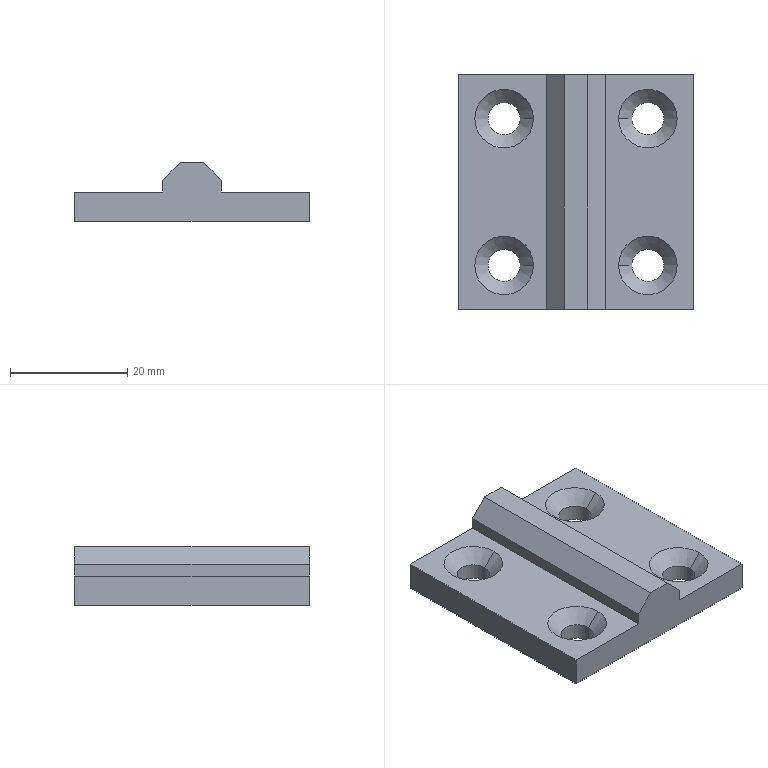Part | STEP file | Hinge bracket 40-40 | 1 solid | 28 faces | box 40 x 40 x 10 mm | volume 8942 mm3 | plane 12 | cone 8 | cylinder 8 | commonest cylinder face diameters 5.5 x8
STEP:
#1=CARTESIAN_POINT('',(-15.,12.5,2.75));
#2=VERTEX_POINT('',#1);
#3=CARTESIAN_POINT('',(-9.5,12.5,2.75));
#4=VERTEX_POINT('',#3);
#5=CARTESIAN_POINT('',(-12.25,12.5,2.75));
#6=DIRECTION('',(0.,0.,1.));
#7=DIRECTION('',(1.,0.,0.));
#8=AXIS2_PLACEMENT_3D('',#5,#6,#7);
#9=CIRCLE('',#8,2.75);
#10=EDGE_CURVE('',#2,#4,#9,.T.);
#11=ORIENTED_EDGE('',*,*,#10,.F.);
#12=CARTESIAN_POINT('',(-17.25,12.5,5.));
#13=VERTEX_POINT('',#12);
#14=CARTESIAN_POINT('',(-17.25,12.5,5.));
#15=DIRECTION('',(-0.7071,0.,0.7071));
#16=VECTOR('',#15,1000.);
#17=LINE('',#14,#16);
#18=EDGE_CURVE('',#2,#13,#17,.T.);
#19=ORIENTED_EDGE('',*,*,#18,.T.);
#20=CARTESIAN_POINT('',(-7.25,12.5,5.));
#21=VERTEX_POINT('',#20);
#22=CARTESIAN_POINT('',(-12.25,12.5,5.));
#23=DIRECTION('',(0.,0.,1.));
#24=DIRECTION('',(1.,0.,0.));
#25=AXIS2_PLACEMENT_3D('',#22,#23,#24);
#26=CIRCLE('',#25,5.);
#27=EDGE_CURVE('',#13,#21,#26,.T.);
#28=ORIENTED_EDGE('',*,*,#27,.T.);
#29=CARTESIAN_POINT('',(-7.25,12.5,5.));
#30=DIRECTION('',(0.7071,0.,0.7071));
#31=VECTOR('',#30,1000.);
#32=LINE('',#29,#31);
#33=EDGE_CURVE('',#4,#21,#32,.T.);
#34=ORIENTED_EDGE('',*,*,#33,.F.);
#35=EDGE_LOOP('',(#11,#19,#28,#34));
#36=FACE_OUTER_BOUND('',#35,.T.);
#37=CARTESIAN_POINT('',(-12.25,12.5,5.));
#38=DIRECTION('',(0.,0.,1.));
#39=DIRECTION('',(1.,0.,0.));
#40=AXIS2_PLACEMENT_3D('',#37,#38,#39);
#41=CONICAL_SURFACE('',#40,5.,0.7854);
#42=ADVANCED_FACE('',(#36),#41,.F.);
#43=CARTESIAN_POINT('',(-15.,12.5,0.));
#44=VERTEX_POINT('',#43);
#45=CARTESIAN_POINT('',(-9.5,12.5,0.));
#46=VERTEX_POINT('',#45);
#47=CARTESIAN_POINT('',(-12.25,12.5,0.));
#48=DIRECTION('',(0.,0.,1.));
#49=DIRECTION('',(1.,0.,0.));
#50=AXIS2_PLACEMENT_3D('',#47,#48,#49);
#51=CIRCLE('',#50,2.75);
#52=EDGE_CURVE('',#44,#46,#51,.T.);
#53=ORIENTED_EDGE('',*,*,#52,.F.);
#54=CARTESIAN_POINT('',(-15.,12.5,5.));
#55=DIRECTION('',(0.,0.,1.));
#56=VECTOR('',#55,1000.);
#57=LINE('',#54,#56);
#58=EDGE_CURVE('',#44,#2,#57,.T.);
#59=ORIENTED_EDGE('',*,*,#58,.T.);
#60=ORIENTED_EDGE('',*,*,#10,.T.);
#61=CARTESIAN_POINT('',(-9.5,12.5,5.));
#62=DIRECTION('',(0.,0.,1.));
#63=VECTOR('',#62,1000.);
#64=LINE('',#61,#63);
#65=EDGE_CURVE('',#46,#4,#64,.T.);
#66=ORIENTED_EDGE('',*,*,#65,.F.);
#67=EDGE_LOOP('',(#53,#59,#60,#66));
#68=FACE_OUTER_BOUND('',#67,.T.);
#69=CARTESIAN_POINT('',(-12.25,12.5,5.));
#70=DIRECTION('',(0.,0.,1.));
#71=DIRECTION('',(1.,0.,0.));
#72=AXIS2_PLACEMENT_3D('',#69,#70,#71);
#73=CYLINDRICAL_SURFACE('',#72,2.75);
#74=ADVANCED_FACE('',(#68),#73,.F.);
#75=CARTESIAN_POINT('',(-15.,-12.5,2.75));
#76=VERTEX_POINT('',#75);
#77=CARTESIAN_POINT('',(-9.5,-12.5,2.75));
#78=VERTEX_POINT('',#77);
#79=CARTESIAN_POINT('',(-12.25,-12.5,2.75));
#80=DIRECTION('',(0.,0.,1.));
#81=DIRECTION('',(1.,0.,0.));
#82=AXIS2_PLACEMENT_3D('',#79,#80,#81);
#83=CIRCLE('',#82,2.75);
#84=EDGE_CURVE('',#76,#78,#83,.T.);
#85=ORIENTED_EDGE('',*,*,#84,.F.);
#86=CARTESIAN_POINT('',(-17.25,-12.5,5.));
#87=VERTEX_POINT('',#86);
#88=CARTESIAN_POINT('',(-17.25,-12.5,5.));
#89=DIRECTION('',(-0.7071,0.,0.7071));
#90=VECTOR('',#89,1000.);
#91=LINE('',#88,#90);
#92=EDGE_CURVE('',#76,#87,#91,.T.);
#93=ORIENTED_EDGE('',*,*,#92,.T.);
#94=CARTESIAN_POINT('',(-7.25,-12.5,5.));
#95=VERTEX_POINT('',#94);
#96=CARTESIAN_POINT('',(-12.25,-12.5,5.));
#97=DIRECTION('',(0.,0.,1.));
#98=DIRECTION('',(1.,0.,0.));
#99=AXIS2_PLACEMENT_3D('',#96,#97,#98);
#100=CIRCLE('',#99,5.);
#101=EDGE_CURVE('',#87,#95,#100,.T.);
#102=ORIENTED_EDGE('',*,*,#101,.T.);
#103=CARTESIAN_POINT('',(-7.25,-12.5,5.));
#104=DIRECTION('',(0.7071,0.,0.7071));
#105=VECTOR('',#104,1000.);
#106=LINE('',#103,#105);
#107=EDGE_CURVE('',#78,#95,#106,.T.);
#108=ORIENTED_EDGE('',*,*,#107,.F.);
#109=EDGE_LOOP('',(#85,#93,#102,#108));
#110=FACE_OUTER_BOUND('',#109,.T.);
#111=CARTESIAN_POINT('',(-12.25,-12.5,5.));
#112=DIRECTION('',(0.,0.,1.));
#113=DIRECTION('',(1.,0.,0.));
#114=AXIS2_PLACEMENT_3D('',#111,#112,#113);
#115=CONICAL_SURFACE('',#114,5.,0.7854);
#116=ADVANCED_FACE('',(#110),#115,.F.);
#117=CARTESIAN_POINT('',(-15.,-12.5,0.));
#118=VERTEX_POINT('',#117);
#119=CARTESIAN_POINT('',(-9.5,-12.5,0.));
#120=VERTEX_POINT('',#119);
#121=CARTESIAN_POINT('',(-12.25,-12.5,0.));
#122=DIRECTION('',(0.,0.,1.));
#123=DIRECTION('',(1.,0.,0.));
#124=AXIS2_PLACEMENT_3D('',#121,#122,#123);
#125=CIRCLE('',#124,2.75);
#126=EDGE_CURVE('',#118,#120,#125,.T.);
#127=ORIENTED_EDGE('',*,*,#126,.F.);
#128=CARTESIAN_POINT('',(-15.,-12.5,5.));
#129=DIRECTION('',(0.,0.,1.));
#130=VECTOR('',#129,1000.);
#131=LINE('',#128,#130);
#132=EDGE_CURVE('',#118,#76,#131,.T.);
#133=ORIENTED_EDGE('',*,*,#132,.T.);
#134=ORIENTED_EDGE('',*,*,#84,.T.);
#135=CARTESIAN_POINT('',(-9.5,-12.5,5.));
#136=DIRECTION('',(0.,0.,1.));
#137=VECTOR('',#136,1000.);
#138=LINE('',#135,#137);
#139=EDGE_CURVE('',#120,#78,#138,.T.);
#140=ORIENTED_EDGE('',*,*,#139,.F.);
#141=EDGE_LOOP('',(#127,#133,#134,#140));
#142=FACE_OUTER_BOUND('',#141,.T.);
#143=CARTESIAN_POINT('',(-12.25,-12.5,5.));
#144=DIRECTION('',(0.,0.,1.));
#145=DIRECTION('',(1.,0.,0.));
#146=AXIS2_PLACEMENT_3D('',#143,#144,#145);
#147=CYLINDRICAL_SURFACE('',#146,2.75);
#148=ADVANCED_FACE('',(#142),#147,.F.);
#149=CARTESIAN_POINT('',(9.5,-12.5,2.75));
#150=VERTEX_POINT('',#149);
#151=CARTESIAN_POINT('',(15.,-12.5,2.75));
#152=VERTEX_POINT('',#151);
#153=CARTESIAN_POINT('',(12.25,-12.5,2.75));
#154=DIRECTION('',(0.,0.,1.));
#155=DIRECTION('',(1.,0.,0.));
#156=AXIS2_PLACEMENT_3D('',#153,#154,#155);
#157=CIRCLE('',#156,2.75);
#158=EDGE_CURVE('',#150,#152,#157,.T.);
#159=ORIENTED_EDGE('',*,*,#158,.F.);
#160=CARTESIAN_POINT('',(7.25,-12.5,5.));
#161=VERTEX_POINT('',#160);
#162=CARTESIAN_POINT('',(7.25,-12.5,5.));
#163=DIRECTION('',(-0.7071,0.,0.7071));
#164=VECTOR('',#163,1000.);
#165=LINE('',#162,#164);
#166=EDGE_CURVE('',#150,#161,#165,.T.);
#167=ORIENTED_EDGE('',*,*,#166,.T.);
#168=CARTESIAN_POINT('',(17.25,-12.5,5.));
#169=VERTEX_POINT('',#168);
#170=CARTESIAN_POINT('',(12.25,-12.5,5.));
#171=DIRECTION('',(0.,0.,1.));
#172=DIRECTION('',(1.,0.,0.));
#173=AXIS2_PLACEMENT_3D('',#170,#171,#172);
#174=CIRCLE('',#173,5.);
#175=EDGE_CURVE('',#161,#169,#174,.T.);
#176=ORIENTED_EDGE('',*,*,#175,.T.);
#177=CARTESIAN_POINT('',(17.25,-12.5,5.));
#178=DIRECTION('',(0.7071,0.,0.7071));
#179=VECTOR('',#178,1000.);
#180=LINE('',#177,#179);
#181=EDGE_CURVE('',#152,#169,#180,.T.);
#182=ORIENTED_EDGE('',*,*,#181,.F.);
#183=EDGE_LOOP('',(#159,#167,#176,#182));
#184=FACE_OUTER_BOUND('',#183,.T.);
#185=CARTESIAN_POINT('',(12.25,-12.5,5.));
#186=DIRECTION('',(0.,0.,1.));
#187=DIRECTION('',(1.,0.,0.));
#188=AXIS2_PLACEMENT_3D('',#185,#186,#187);
#189=CONICAL_SURFACE('',#188,5.,0.7854);
#190=ADVANCED_FACE('',(#184),#189,.F.);
#191=CARTESIAN_POINT('',(9.5,-12.5,0.));
#192=VERTEX_POINT('',#191);
#193=CARTESIAN_POINT('',(15.,-12.5,0.));
#194=VERTEX_POINT('',#193);
#195=CARTESIAN_POINT('',(12.25,-12.5,0.));
#196=DIRECTION('',(0.,0.,1.));
#197=DIRECTION('',(1.,0.,0.));
#198=AXIS2_PLACEMENT_3D('',#195,#196,#197);
#199=CIRCLE('',#198,2.75);
#200=EDGE_CURVE('',#192,#194,#199,.T.);
#201=ORIENTED_EDGE('',*,*,#200,.F.);
#202=CARTESIAN_POINT('',(9.5,-12.5,5.));
#203=DIRECTION('',(0.,0.,1.));
#204=VECTOR('',#203,1000.);
#205=LINE('',#202,#204);
#206=EDGE_CURVE('',#192,#150,#205,.T.);
#207=ORIENTED_EDGE('',*,*,#206,.T.);
#208=ORIENTED_EDGE('',*,*,#158,.T.);
#209=CARTESIAN_POINT('',(15.,-12.5,5.));
#210=DIRECTION('',(0.,0.,1.));
#211=VECTOR('',#210,1000.);
#212=LINE('',#209,#211);
#213=EDGE_CURVE('',#194,#152,#212,.T.);
#214=ORIENTED_EDGE('',*,*,#213,.F.);
#215=EDGE_LOOP('',(#201,#207,#208,#214));
#216=FACE_OUTER_BOUND('',#215,.T.);
#217=CARTESIAN_POINT('',(12.25,-12.5,5.));
#218=DIRECTION('',(0.,0.,1.));
#219=DIRECTION('',(1.,0.,0.));
#220=AXIS2_PLACEMENT_3D('',#217,#218,#219);
#221=CYLINDRICAL_SURFACE('',#220,2.75);
#222=ADVANCED_FACE('',(#216),#221,.F.);
#223=CARTESIAN_POINT('',(9.5,12.5,2.75));
#224=VERTEX_POINT('',#223);
#225=CARTESIAN_POINT('',(15.,12.5,2.75));
#226=VERTEX_POINT('',#225);
#227=CARTESIAN_POINT('',(12.25,12.5,2.75));
#228=DIRECTION('',(0.,0.,1.));
#229=DIRECTION('',(1.,0.,0.));
#230=AXIS2_PLACEMENT_3D('',#227,#228,#229);
#231=CIRCLE('',#230,2.75);
#232=EDGE_CURVE('',#224,#226,#231,.T.);
#233=ORIENTED_EDGE('',*,*,#232,.F.);
#234=CARTESIAN_POINT('',(7.25,12.5,5.));
#235=VERTEX_POINT('',#234);
#236=CARTESIAN_POINT('',(7.25,12.5,5.));
#237=DIRECTION('',(-0.7071,0.,0.7071));
#238=VECTOR('',#237,1000.);
#239=LINE('',#236,#238);
#240=EDGE_CURVE('',#224,#235,#239,.T.);
#241=ORIENTED_EDGE('',*,*,#240,.T.);
#242=CARTESIAN_POINT('',(17.25,12.5,5.));
#243=VERTEX_POINT('',#242);
#244=CARTESIAN_POINT('',(12.25,12.5,5.));
#245=DIRECTION('',(0.,0.,1.));
#246=DIRECTION('',(1.,0.,0.));
#247=AXIS2_PLACEMENT_3D('',#244,#245,#246);
#248=CIRCLE('',#247,5.);
#249=EDGE_CURVE('',#235,#243,#248,.T.);
#250=ORIENTED_EDGE('',*,*,#249,.T.);
#251=CARTESIAN_POINT('',(17.25,12.5,5.));
#252=DIRECTION('',(0.7071,0.,0.7071));
#253=VECTOR('',#252,1000.);
#254=LINE('',#251,#253);
#255=EDGE_CURVE('',#226,#243,#254,.T.);
#256=ORIENTED_EDGE('',*,*,#255,.F.);
#257=EDGE_LOOP('',(#233,#241,#250,#256));
#258=FACE_OUTER_BOUND('',#257,.T.);
#259=CARTESIAN_POINT('',(12.25,12.5,5.));
#260=DIRECTION('',(0.,0.,1.));
#261=DIRECTION('',(1.,0.,0.));
#262=AXIS2_PLACEMENT_3D('',#259,#260,#261);
#263=CONICAL_SURFACE('',#262,5.,0.7854);
#264=ADVANCED_FACE('',(#258),#263,.F.);
#265=CARTESIAN_POINT('',(9.5,12.5,0.));
#266=VERTEX_POINT('',#265);
#267=CARTESIAN_POINT('',(15.,12.5,0.));
#268=VERTEX_POINT('',#267);
#269=CARTESIAN_POINT('',(12.25,12.5,0.));
#270=DIRECTION('',(0.,0.,1.));
#271=DIRECTION('',(1.,0.,0.));
#272=AXIS2_PLACEMENT_3D('',#269,#270,#271);
#273=CIRCLE('',#272,2.75);
#274=EDGE_CURVE('',#266,#268,#273,.T.);
#275=ORIENTED_EDGE('',*,*,#274,.F.);
#276=CARTESIAN_POINT('',(9.5,12.5,5.));
#277=DIRECTION('',(0.,0.,1.));
#278=VECTOR('',#277,1000.);
#279=LINE('',#276,#278);
#280=EDGE_CURVE('',#266,#224,#279,.T.);
#281=ORIENTED_EDGE('',*,*,#280,.T.);
#282=ORIENTED_EDGE('',*,*,#232,.T.);
#283=CARTESIAN_POINT('',(15.,12.5,5.));
#284=DIRECTION('',(0.,0.,1.));
#285=VECTOR('',#284,1000.);
#286=LINE('',#283,#285);
#287=EDGE_CURVE('',#268,#226,#286,.T.);
#288=ORIENTED_EDGE('',*,*,#287,.F.);
#289=EDGE_LOOP('',(#275,#281,#282,#288));
#290=FACE_OUTER_BOUND('',#289,.T.);
#291=CARTESIAN_POINT('',(12.25,12.5,5.));
#292=DIRECTION('',(0.,0.,1.));
#293=DIRECTION('',(1.,0.,0.));
#294=AXIS2_PLACEMENT_3D('',#291,#292,#293);
#295=CYLINDRICAL_SURFACE('',#294,2.75);
#296=ADVANCED_FACE('',(#290),#295,.F.);
#297=CARTESIAN_POINT('',(12.25,-12.5,5.));
#298=DIRECTION('',(0.,0.,1.));
#299=DIRECTION('',(1.,0.,0.));
#300=AXIS2_PLACEMENT_3D('',#297,#298,#299);
#301=CIRCLE('',#300,5.);
#302=EDGE_CURVE('',#169,#161,#301,.T.);
#303=ORIENTED_EDGE('',*,*,#302,.F.);
#304=ORIENTED_EDGE('',*,*,#175,.F.);
#305=EDGE_LOOP('',(#303,#304));
#306=FACE_BOUND('',#305,.T.);
#307=CARTESIAN_POINT('',(12.25,12.5,5.));
#308=DIRECTION('',(0.,0.,1.));
#309=DIRECTION('',(1.,0.,0.));
#310=AXIS2_PLACEMENT_3D('',#307,#308,#309);
#311=CIRCLE('',#310,5.);
#312=EDGE_CURVE('',#243,#235,#311,.T.);
#313=ORIENTED_EDGE('',*,*,#312,.F.);
#314=ORIENTED_EDGE('',*,*,#249,.F.);
#315=EDGE_LOOP('',(#313,#314));
#316=FACE_BOUND('',#315,.T.);
#317=CARTESIAN_POINT('',(5.,-20.,5.));
#318=VERTEX_POINT('',#317);
#319=CARTESIAN_POINT('',(5.,20.,5.));
#320=VERTEX_POINT('',#319);
#321=CARTESIAN_POINT('',(5.,-20.,5.));
#322=DIRECTION('',(0.,1.,0.));
#323=VECTOR('',#322,1000.);
#324=LINE('',#321,#323);
#325=EDGE_CURVE('',#318,#320,#324,.T.);
#326=ORIENTED_EDGE('',*,*,#325,.F.);
#327=CARTESIAN_POINT('',(20.,-20.,5.));
#328=VERTEX_POINT('',#327);
#329=CARTESIAN_POINT('',(-20.,-20.,5.));
#330=DIRECTION('',(1.,0.,0.));
#331=VECTOR('',#330,1000.);
#332=LINE('',#329,#331);
#333=EDGE_CURVE('',#318,#328,#332,.T.);
#334=ORIENTED_EDGE('',*,*,#333,.T.);
#335=CARTESIAN_POINT('',(20.,20.,5.));
#336=VERTEX_POINT('',#335);
#337=CARTESIAN_POINT('',(20.,-20.,5.));
#338=DIRECTION('',(0.,1.,0.));
#339=VECTOR('',#338,1000.);
#340=LINE('',#337,#339);
#341=EDGE_CURVE('',#328,#336,#340,.T.);
#342=ORIENTED_EDGE('',*,*,#341,.T.);
#343=CARTESIAN_POINT('',(-20.,20.,5.));
#344=DIRECTION('',(-1.,0.,0.));
#345=VECTOR('',#344,1000.);
#346=LINE('',#343,#345);
#347=EDGE_CURVE('',#336,#320,#346,.T.);
#348=ORIENTED_EDGE('',*,*,#347,.T.);
#349=EDGE_LOOP('',(#326,#334,#342,#348));
#350=FACE_OUTER_BOUND('',#349,.T.);
#351=CARTESIAN_POINT('',(20.,20.,5.));
#352=DIRECTION('',(0.,0.,-1.));
#353=DIRECTION('',(-1.,0.,0.));
#354=AXIS2_PLACEMENT_3D('',#351,#352,#353);
#355=PLANE('',#354);
#356=ADVANCED_FACE('',(#306,#316,#350),#355,.F.);
#357=CARTESIAN_POINT('',(20.,-20.,0.));
#358=VERTEX_POINT('',#357);
#359=CARTESIAN_POINT('',(20.,20.,0.));
#360=VERTEX_POINT('',#359);
#361=CARTESIAN_POINT('',(20.,-20.,0.));
#362=DIRECTION('',(0.,1.,0.));
#363=VECTOR('',#362,1000.);
#364=LINE('',#361,#363);
#365=EDGE_CURVE('',#358,#360,#364,.T.);
#366=ORIENTED_EDGE('',*,*,#365,.T.);
#367=CARTESIAN_POINT('',(20.,20.,5.));
#368=DIRECTION('',(0.,0.,-1.));
#369=VECTOR('',#368,1000.);
#370=LINE('',#367,#369);
#371=EDGE_CURVE('',#336,#360,#370,.T.);
#372=ORIENTED_EDGE('',*,*,#371,.F.);
#373=ORIENTED_EDGE('',*,*,#341,.F.);
#374=CARTESIAN_POINT('',(20.,-20.,5.));
#375=DIRECTION('',(0.,0.,-1.));
#376=VECTOR('',#375,1000.);
#377=LINE('',#374,#376);
#378=EDGE_CURVE('',#328,#358,#377,.T.);
#379=ORIENTED_EDGE('',*,*,#378,.T.);
#380=EDGE_LOOP('',(#366,#372,#373,#379));
#381=FACE_OUTER_BOUND('',#380,.T.);
#382=CARTESIAN_POINT('',(20.,-20.,5.));
#383=DIRECTION('',(-1.,0.,0.));
#384=DIRECTION('',(0.,0.,1.));
#385=AXIS2_PLACEMENT_3D('',#382,#383,#384);
#386=PLANE('',#385);
#387=ADVANCED_FACE('',(#381),#386,.F.);
#388=CARTESIAN_POINT('',(-2.,20.,10.));
#389=VERTEX_POINT('',#388);
#390=CARTESIAN_POINT('',(2.,20.,10.));
#391=VERTEX_POINT('',#390);
#392=CARTESIAN_POINT('',(-5.,20.,10.));
#393=DIRECTION('',(1.,0.,0.));
#394=VECTOR('',#393,1000.);
#395=LINE('',#392,#394);
#396=EDGE_CURVE('',#389,#391,#395,.T.);
#397=ORIENTED_EDGE('',*,*,#396,.T.);
#398=CARTESIAN_POINT('',(5.,20.,7.));
#399=VERTEX_POINT('',#398);
#400=CARTESIAN_POINT('',(2.,20.,10.));
#401=DIRECTION('',(0.7071,0.,-0.7071));
#402=VECTOR('',#401,1000.);
#403=LINE('',#400,#402);
#404=EDGE_CURVE('',#391,#399,#403,.T.);
#405=ORIENTED_EDGE('',*,*,#404,.T.);
#406=CARTESIAN_POINT('',(5.,20.,5.));
#407=DIRECTION('',(0.,0.,-1.));
#408=VECTOR('',#407,1000.);
#409=LINE('',#406,#408);
#410=EDGE_CURVE('',#399,#320,#409,.T.);
#411=ORIENTED_EDGE('',*,*,#410,.T.);
#412=ORIENTED_EDGE('',*,*,#347,.F.);
#413=ORIENTED_EDGE('',*,*,#371,.T.);
#414=CARTESIAN_POINT('',(-20.,20.,0.));
#415=VERTEX_POINT('',#414);
#416=CARTESIAN_POINT('',(-20.,20.,0.));
#417=DIRECTION('',(-1.,0.,0.));
#418=VECTOR('',#417,1000.);
#419=LINE('',#416,#418);
#420=EDGE_CURVE('',#360,#415,#419,.T.);
#421=ORIENTED_EDGE('',*,*,#420,.T.);
#422=CARTESIAN_POINT('',(-20.,20.,5.));
#423=VERTEX_POINT('',#422);
#424=CARTESIAN_POINT('',(-20.,20.,5.));
#425=DIRECTION('',(0.,0.,-1.));
#426=VECTOR('',#425,1000.);
#427=LINE('',#424,#426);
#428=EDGE_CURVE('',#423,#415,#427,.T.);
#429=ORIENTED_EDGE('',*,*,#428,.F.);
#430=CARTESIAN_POINT('',(-5.,20.,5.));
#431=VERTEX_POINT('',#430);
#432=CARTESIAN_POINT('',(-20.,20.,5.));
#433=DIRECTION('',(-1.,0.,0.));
#434=VECTOR('',#433,1000.);
#435=LINE('',#432,#434);
#436=EDGE_CURVE('',#431,#423,#435,.T.);
#437=ORIENTED_EDGE('',*,*,#436,.F.);
#438=CARTESIAN_POINT('',(-5.,20.,7.));
#439=VERTEX_POINT('',#438);
#440=CARTESIAN_POINT('',(-5.,20.,5.));
#441=DIRECTION('',(0.,0.,1.));
#442=VECTOR('',#441,1000.);
#443=LINE('',#440,#442);
#444=EDGE_CURVE('',#431,#439,#443,.T.);
#445=ORIENTED_EDGE('',*,*,#444,.T.);
#446=CARTESIAN_POINT('',(-5.,20.,7.));
#447=DIRECTION('',(0.7071,0.,0.7071));
#448=VECTOR('',#447,1000.);
#449=LINE('',#446,#448);
#450=EDGE_CURVE('',#439,#389,#449,.T.);
#451=ORIENTED_EDGE('',*,*,#450,.T.);
#452=EDGE_LOOP('',(#397,#405,#411,#412,#413,#421,#429,#437,#445,#451));
#453=FACE_OUTER_BOUND('',#452,.T.);
#454=CARTESIAN_POINT('',(-20.,20.,5.));
#455=DIRECTION('',(0.,-1.,0.));
#456=DIRECTION('',(0.,0.,-1.));
#457=AXIS2_PLACEMENT_3D('',#454,#455,#456);
#458=PLANE('',#457);
#459=ADVANCED_FACE('',(#453),#458,.F.);
#460=CARTESIAN_POINT('',(-20.,-20.,0.));
#461=VERTEX_POINT('',#460);
#462=CARTESIAN_POINT('',(-20.,-20.,0.));
#463=DIRECTION('',(0.,-1.,0.));
#464=VECTOR('',#463,1000.);
#465=LINE('',#462,#464);
#466=EDGE_CURVE('',#415,#461,#465,.T.);
#467=ORIENTED_EDGE('',*,*,#466,.T.);
#468=CARTESIAN_POINT('',(-20.,-20.,5.));
#469=VERTEX_POINT('',#468);
#470=CARTESIAN_POINT('',(-20.,-20.,5.));
#471=DIRECTION('',(0.,0.,-1.));
#472=VECTOR('',#471,1000.);
#473=LINE('',#470,#472);
#474=EDGE_CURVE('',#469,#461,#473,.T.);
#475=ORIENTED_EDGE('',*,*,#474,.F.);
#476=CARTESIAN_POINT('',(-20.,-20.,5.));
#477=DIRECTION('',(0.,-1.,0.));
#478=VECTOR('',#477,1000.);
#479=LINE('',#476,#478);
#480=EDGE_CURVE('',#423,#469,#479,.T.);
#481=ORIENTED_EDGE('',*,*,#480,.F.);
#482=ORIENTED_EDGE('',*,*,#428,.T.);
#483=EDGE_LOOP('',(#467,#475,#481,#482));
#484=FACE_OUTER_BOUND('',#483,.T.);
#485=CARTESIAN_POINT('',(-20.,-20.,5.));
#486=DIRECTION('',(1.,0.,0.));
#487=DIRECTION('',(0.,0.,-1.));
#488=AXIS2_PLACEMENT_3D('',#485,#486,#487);
#489=PLANE('',#488);
#490=ADVANCED_FACE('',(#484),#489,.F.);
#491=CARTESIAN_POINT('',(5.,-20.,7.));
#492=VERTEX_POINT('',#491);
#493=CARTESIAN_POINT('',(5.,-20.,5.));
#494=DIRECTION('',(0.,0.,-1.));
#495=VECTOR('',#494,1000.);
#496=LINE('',#493,#495);
#497=EDGE_CURVE('',#492,#318,#496,.T.);
#498=ORIENTED_EDGE('',*,*,#497,.F.);
#499=CARTESIAN_POINT('',(2.,-20.,10.));
#500=VERTEX_POINT('',#499);
#501=CARTESIAN_POINT('',(2.,-20.,10.));
#502=DIRECTION('',(-0.7071,0.,0.7071));
#503=VECTOR('',#502,1000.);
#504=LINE('',#501,#503);
#505=EDGE_CURVE('',#492,#500,#504,.T.);
#506=ORIENTED_EDGE('',*,*,#505,.T.);
#507=CARTESIAN_POINT('',(-2.,-20.,10.));
#508=VERTEX_POINT('',#507);
#509=CARTESIAN_POINT('',(-5.,-20.,10.));
#510=DIRECTION('',(1.,0.,0.));
#511=VECTOR('',#510,1000.);
#512=LINE('',#509,#511);
#513=EDGE_CURVE('',#508,#500,#512,.T.);
#514=ORIENTED_EDGE('',*,*,#513,.F.);
#515=CARTESIAN_POINT('',(-5.,-20.,7.));
#516=VERTEX_POINT('',#515);
#517=CARTESIAN_POINT('',(-5.,-20.,7.));
#518=DIRECTION('',(-0.7071,0.,-0.7071));
#519=VECTOR('',#518,1000.);
#520=LINE('',#517,#519);
#521=EDGE_CURVE('',#508,#516,#520,.T.);
#522=ORIENTED_EDGE('',*,*,#521,.T.);
#523=CARTESIAN_POINT('',(-5.,-20.,5.));
#524=VERTEX_POINT('',#523);
#525=CARTESIAN_POINT('',(-5.,-20.,5.));
#526=DIRECTION('',(0.,0.,1.));
#527=VECTOR('',#526,1000.);
#528=LINE('',#525,#527);
#529=EDGE_CURVE('',#524,#516,#528,.T.);
#530=ORIENTED_EDGE('',*,*,#529,.F.);
#531=CARTESIAN_POINT('',(-20.,-20.,5.));
#532=DIRECTION('',(1.,0.,0.));
#533=VECTOR('',#532,1000.);
#534=LINE('',#531,#533);
#535=EDGE_CURVE('',#469,#524,#534,.T.);
#536=ORIENTED_EDGE('',*,*,#535,.F.);
#537=ORIENTED_EDGE('',*,*,#474,.T.);
#538=CARTESIAN_POINT('',(-20.,-20.,0.));
#539=DIRECTION('',(1.,0.,0.));
#540=VECTOR('',#539,1000.);
#541=LINE('',#538,#540);
#542=EDGE_CURVE('',#461,#358,#541,.T.);
#543=ORIENTED_EDGE('',*,*,#542,.T.);
#544=ORIENTED_EDGE('',*,*,#378,.F.);
#545=ORIENTED_EDGE('',*,*,#333,.F.);
#546=EDGE_LOOP('',(#498,#506,#514,#522,#530,#536,#537,#543,#544,#545));
#547=FACE_OUTER_BOUND('',#546,.T.);
#548=CARTESIAN_POINT('',(-20.,-20.,5.));
#549=DIRECTION('',(0.,1.,0.));
#550=DIRECTION('',(0.,0.,1.));
#551=AXIS2_PLACEMENT_3D('',#548,#549,#550);
#552=PLANE('',#551);
#553=ADVANCED_FACE('',(#547),#552,.F.);
#554=CARTESIAN_POINT('',(-12.25,12.5,5.));
#555=DIRECTION('',(0.,0.,1.));
#556=DIRECTION('',(1.,0.,0.));
#557=AXIS2_PLACEMENT_3D('',#554,#555,#556);
#558=CIRCLE('',#557,5.);
#559=EDGE_CURVE('',#21,#13,#558,.T.);
#560=ORIENTED_EDGE('',*,*,#559,.F.);
#561=ORIENTED_EDGE('',*,*,#27,.F.);
#562=EDGE_LOOP('',(#560,#561));
#563=FACE_BOUND('',#562,.T.);
#564=CARTESIAN_POINT('',(-12.25,-12.5,5.));
#565=DIRECTION('',(0.,0.,1.));
#566=DIRECTION('',(1.,0.,0.));
#567=AXIS2_PLACEMENT_3D('',#564,#565,#566);
#568=CIRCLE('',#567,5.);
#569=EDGE_CURVE('',#95,#87,#568,.T.);
#570=ORIENTED_EDGE('',*,*,#569,.F.);
#571=ORIENTED_EDGE('',*,*,#101,.F.);
#572=EDGE_LOOP('',(#570,#571));
#573=FACE_BOUND('',#572,.T.);
#574=ORIENTED_EDGE('',*,*,#535,.T.);
#575=CARTESIAN_POINT('',(-5.,-20.,5.));
#576=DIRECTION('',(0.,1.,0.));
#577=VECTOR('',#576,1000.);
#578=LINE('',#575,#577);
#579=EDGE_CURVE('',#524,#431,#578,.T.);
#580=ORIENTED_EDGE('',*,*,#579,.T.);
#581=ORIENTED_EDGE('',*,*,#436,.T.);
#582=ORIENTED_EDGE('',*,*,#480,.T.);
#583=EDGE_LOOP('',(#574,#580,#581,#582));
#584=FACE_OUTER_BOUND('',#583,.T.);
#585=CARTESIAN_POINT('',(20.,20.,5.));
#586=DIRECTION('',(0.,0.,-1.));
#587=DIRECTION('',(-1.,0.,0.));
#588=AXIS2_PLACEMENT_3D('',#585,#586,#587);
#589=PLANE('',#588);
#590=ADVANCED_FACE('',(#563,#573,#584),#589,.F.);
#591=CARTESIAN_POINT('',(-12.25,12.5,0.));
#592=DIRECTION('',(0.,0.,1.));
#593=DIRECTION('',(1.,0.,0.));
#594=AXIS2_PLACEMENT_3D('',#591,#592,#593);
#595=CIRCLE('',#594,2.75);
#596=EDGE_CURVE('',#46,#44,#595,.T.);
#597=ORIENTED_EDGE('',*,*,#596,.T.);
#598=ORIENTED_EDGE('',*,*,#52,.T.);
#599=EDGE_LOOP('',(#597,#598));
#600=FACE_BOUND('',#599,.T.);
#601=CARTESIAN_POINT('',(-12.25,-12.5,0.));
#602=DIRECTION('',(0.,0.,1.));
#603=DIRECTION('',(1.,0.,0.));
#604=AXIS2_PLACEMENT_3D('',#601,#602,#603);
#605=CIRCLE('',#604,2.75);
#606=EDGE_CURVE('',#120,#118,#605,.T.);
#607=ORIENTED_EDGE('',*,*,#606,.T.);
#608=ORIENTED_EDGE('',*,*,#126,.T.);
#609=EDGE_LOOP('',(#607,#608));
#610=FACE_BOUND('',#609,.T.);
#611=CARTESIAN_POINT('',(12.25,-12.5,0.));
#612=DIRECTION('',(0.,0.,1.));
#613=DIRECTION('',(1.,0.,0.));
#614=AXIS2_PLACEMENT_3D('',#611,#612,#613);
#615=CIRCLE('',#614,2.75);
#616=EDGE_CURVE('',#194,#192,#615,.T.);
#617=ORIENTED_EDGE('',*,*,#616,.T.);
#618=ORIENTED_EDGE('',*,*,#200,.T.);
#619=EDGE_LOOP('',(#617,#618));
#620=FACE_BOUND('',#619,.T.);
#621=CARTESIAN_POINT('',(12.25,12.5,0.));
#622=DIRECTION('',(0.,0.,1.));
#623=DIRECTION('',(1.,0.,0.));
#624=AXIS2_PLACEMENT_3D('',#621,#622,#623);
#625=CIRCLE('',#624,2.75);
#626=EDGE_CURVE('',#268,#266,#625,.T.);
#627=ORIENTED_EDGE('',*,*,#626,.T.);
#628=ORIENTED_EDGE('',*,*,#274,.T.);
#629=EDGE_LOOP('',(#627,#628));
#630=FACE_BOUND('',#629,.T.);
#631=ORIENTED_EDGE('',*,*,#365,.F.);
#632=ORIENTED_EDGE('',*,*,#542,.F.);
#633=ORIENTED_EDGE('',*,*,#466,.F.);
#634=ORIENTED_EDGE('',*,*,#420,.F.);
#635=EDGE_LOOP('',(#631,#632,#633,#634));
#636=FACE_OUTER_BOUND('',#635,.T.);
#637=CARTESIAN_POINT('',(20.,20.,0.));
#638=DIRECTION('',(0.,0.,-1.));
#639=DIRECTION('',(-1.,0.,0.));
#640=AXIS2_PLACEMENT_3D('',#637,#638,#639);
#641=PLANE('',#640);
#642=ADVANCED_FACE('',(#600,#610,#620,#630,#636),#641,.T.);
#643=ORIENTED_EDGE('',*,*,#280,.F.);
#644=ORIENTED_EDGE('',*,*,#626,.F.);
#645=ORIENTED_EDGE('',*,*,#287,.T.);
#646=CARTESIAN_POINT('',(12.25,12.5,2.75));
#647=DIRECTION('',(0.,0.,1.));
#648=DIRECTION('',(1.,0.,0.));
#649=AXIS2_PLACEMENT_3D('',#646,#647,#648);
#650=CIRCLE('',#649,2.75);
#651=EDGE_CURVE('',#226,#224,#650,.T.);
#652=ORIENTED_EDGE('',*,*,#651,.T.);
#653=EDGE_LOOP('',(#643,#644,#645,#652));
#654=FACE_OUTER_BOUND('',#653,.T.);
#655=CARTESIAN_POINT('',(12.25,12.5,5.));
#656=DIRECTION('',(0.,0.,1.));
#657=DIRECTION('',(1.,0.,0.));
#658=AXIS2_PLACEMENT_3D('',#655,#656,#657);
#659=CYLINDRICAL_SURFACE('',#658,2.75);
#660=ADVANCED_FACE('',(#654),#659,.F.);
#661=ORIENTED_EDGE('',*,*,#240,.F.);
#662=ORIENTED_EDGE('',*,*,#651,.F.);
#663=ORIENTED_EDGE('',*,*,#255,.T.);
#664=ORIENTED_EDGE('',*,*,#312,.T.);
#665=EDGE_LOOP('',(#661,#662,#663,#664));
#666=FACE_OUTER_BOUND('',#665,.T.);
#667=CARTESIAN_POINT('',(12.25,12.5,5.));
#668=DIRECTION('',(0.,0.,1.));
#669=DIRECTION('',(1.,0.,0.));
#670=AXIS2_PLACEMENT_3D('',#667,#668,#669);
#671=CONICAL_SURFACE('',#670,5.,0.7854);
#672=ADVANCED_FACE('',(#666),#671,.F.);
#673=ORIENTED_EDGE('',*,*,#206,.F.);
#674=ORIENTED_EDGE('',*,*,#616,.F.);
#675=ORIENTED_EDGE('',*,*,#213,.T.);
#676=CARTESIAN_POINT('',(12.25,-12.5,2.75));
#677=DIRECTION('',(0.,0.,1.));
#678=DIRECTION('',(1.,0.,0.));
#679=AXIS2_PLACEMENT_3D('',#676,#677,#678);
#680=CIRCLE('',#679,2.75);
#681=EDGE_CURVE('',#152,#150,#680,.T.);
#682=ORIENTED_EDGE('',*,*,#681,.T.);
#683=EDGE_LOOP('',(#673,#674,#675,#682));
#684=FACE_OUTER_BOUND('',#683,.T.);
#685=CARTESIAN_POINT('',(12.25,-12.5,5.));
#686=DIRECTION('',(0.,0.,1.));
#687=DIRECTION('',(1.,0.,0.));
#688=AXIS2_PLACEMENT_3D('',#685,#686,#687);
#689=CYLINDRICAL_SURFACE('',#688,2.75);
#690=ADVANCED_FACE('',(#684),#689,.F.);
#691=ORIENTED_EDGE('',*,*,#166,.F.);
#692=ORIENTED_EDGE('',*,*,#681,.F.);
#693=ORIENTED_EDGE('',*,*,#181,.T.);
#694=ORIENTED_EDGE('',*,*,#302,.T.);
#695=EDGE_LOOP('',(#691,#692,#693,#694));
#696=FACE_OUTER_BOUND('',#695,.T.);
#697=CARTESIAN_POINT('',(12.25,-12.5,5.));
#698=DIRECTION('',(0.,0.,1.));
#699=DIRECTION('',(1.,0.,0.));
#700=AXIS2_PLACEMENT_3D('',#697,#698,#699);
#701=CONICAL_SURFACE('',#700,5.,0.7854);
#702=ADVANCED_FACE('',(#696),#701,.F.);
#703=ORIENTED_EDGE('',*,*,#132,.F.);
#704=ORIENTED_EDGE('',*,*,#606,.F.);
#705=ORIENTED_EDGE('',*,*,#139,.T.);
#706=CARTESIAN_POINT('',(-12.25,-12.5,2.75));
#707=DIRECTION('',(0.,0.,1.));
#708=DIRECTION('',(1.,0.,0.));
#709=AXIS2_PLACEMENT_3D('',#706,#707,#708);
#710=CIRCLE('',#709,2.75);
#711=EDGE_CURVE('',#78,#76,#710,.T.);
#712=ORIENTED_EDGE('',*,*,#711,.T.);
#713=EDGE_LOOP('',(#703,#704,#705,#712));
#714=FACE_OUTER_BOUND('',#713,.T.);
#715=CARTESIAN_POINT('',(-12.25,-12.5,5.));
#716=DIRECTION('',(0.,0.,1.));
#717=DIRECTION('',(1.,0.,0.));
#718=AXIS2_PLACEMENT_3D('',#715,#716,#717);
#719=CYLINDRICAL_SURFACE('',#718,2.75);
#720=ADVANCED_FACE('',(#714),#719,.F.);
#721=ORIENTED_EDGE('',*,*,#92,.F.);
#722=ORIENTED_EDGE('',*,*,#711,.F.);
#723=ORIENTED_EDGE('',*,*,#107,.T.);
#724=ORIENTED_EDGE('',*,*,#569,.T.);
#725=EDGE_LOOP('',(#721,#722,#723,#724));
#726=FACE_OUTER_BOUND('',#725,.T.);
#727=CARTESIAN_POINT('',(-12.25,-12.5,5.));
#728=DIRECTION('',(0.,0.,1.));
#729=DIRECTION('',(1.,0.,0.));
#730=AXIS2_PLACEMENT_3D('',#727,#728,#729);
#731=CONICAL_SURFACE('',#730,5.,0.7854);
#732=ADVANCED_FACE('',(#726),#731,.F.);
#733=ORIENTED_EDGE('',*,*,#58,.F.);
#734=ORIENTED_EDGE('',*,*,#596,.F.);
#735=ORIENTED_EDGE('',*,*,#65,.T.);
#736=CARTESIAN_POINT('',(-12.25,12.5,2.75));
#737=DIRECTION('',(0.,0.,1.));
#738=DIRECTION('',(1.,0.,0.));
#739=AXIS2_PLACEMENT_3D('',#736,#737,#738);
#740=CIRCLE('',#739,2.75);
#741=EDGE_CURVE('',#4,#2,#740,.T.);
#742=ORIENTED_EDGE('',*,*,#741,.T.);
#743=EDGE_LOOP('',(#733,#734,#735,#742));
#744=FACE_OUTER_BOUND('',#743,.T.);
#745=CARTESIAN_POINT('',(-12.25,12.5,5.));
#746=DIRECTION('',(0.,0.,1.));
#747=DIRECTION('',(1.,0.,0.));
#748=AXIS2_PLACEMENT_3D('',#745,#746,#747);
#749=CYLINDRICAL_SURFACE('',#748,2.75);
#750=ADVANCED_FACE('',(#744),#749,.F.);
#751=ORIENTED_EDGE('',*,*,#18,.F.);
#752=ORIENTED_EDGE('',*,*,#741,.F.);
#753=ORIENTED_EDGE('',*,*,#33,.T.);
#754=ORIENTED_EDGE('',*,*,#559,.T.);
#755=EDGE_LOOP('',(#751,#752,#753,#754));
#756=FACE_OUTER_BOUND('',#755,.T.);
#757=CARTESIAN_POINT('',(-12.25,12.5,5.));
#758=DIRECTION('',(0.,0.,1.));
#759=DIRECTION('',(1.,0.,0.));
#760=AXIS2_PLACEMENT_3D('',#757,#758,#759);
#761=CONICAL_SURFACE('',#760,5.,0.7854);
#762=ADVANCED_FACE('',(#756),#761,.F.);
#763=ORIENTED_EDGE('',*,*,#410,.F.);
#764=CARTESIAN_POINT('',(5.,-20.,7.));
#765=DIRECTION('',(0.,-1.,0.));
#766=VECTOR('',#765,1000.);
#767=LINE('',#764,#766);
#768=EDGE_CURVE('',#399,#492,#767,.T.);
#769=ORIENTED_EDGE('',*,*,#768,.T.);
#770=ORIENTED_EDGE('',*,*,#497,.T.);
#771=ORIENTED_EDGE('',*,*,#325,.T.);
#772=EDGE_LOOP('',(#763,#769,#770,#771));
#773=FACE_OUTER_BOUND('',#772,.T.);
#774=CARTESIAN_POINT('',(5.,-20.,5.));
#775=DIRECTION('',(1.,0.,0.));
#776=DIRECTION('',(0.,0.,-1.));
#777=AXIS2_PLACEMENT_3D('',#774,#775,#776);
#778=PLANE('',#777);
#779=ADVANCED_FACE('',(#773),#778,.T.);
#780=ORIENTED_EDGE('',*,*,#513,.T.);
#781=CARTESIAN_POINT('',(2.,-20.,10.));
#782=DIRECTION('',(0.,1.,0.));
#783=VECTOR('',#782,1000.);
#784=LINE('',#781,#783);
#785=EDGE_CURVE('',#500,#391,#784,.T.);
#786=ORIENTED_EDGE('',*,*,#785,.T.);
#787=ORIENTED_EDGE('',*,*,#396,.F.);
#788=CARTESIAN_POINT('',(-2.,-20.,10.));
#789=DIRECTION('',(0.,-1.,0.));
#790=VECTOR('',#789,1000.);
#791=LINE('',#788,#790);
#792=EDGE_CURVE('',#389,#508,#791,.T.);
#793=ORIENTED_EDGE('',*,*,#792,.T.);
#794=EDGE_LOOP('',(#780,#786,#787,#793));
#795=FACE_OUTER_BOUND('',#794,.T.);
#796=CARTESIAN_POINT('',(-5.,-20.,10.));
#797=DIRECTION('',(0.,0.,1.));
#798=DIRECTION('',(1.,0.,0.));
#799=AXIS2_PLACEMENT_3D('',#796,#797,#798);
#800=PLANE('',#799);
#801=ADVANCED_FACE('',(#795),#800,.T.);
#802=ORIENTED_EDGE('',*,*,#529,.T.);
#803=CARTESIAN_POINT('',(-5.,-20.,7.));
#804=DIRECTION('',(0.,1.,0.));
#805=VECTOR('',#804,1000.);
#806=LINE('',#803,#805);
#807=EDGE_CURVE('',#516,#439,#806,.T.);
#808=ORIENTED_EDGE('',*,*,#807,.T.);
#809=ORIENTED_EDGE('',*,*,#444,.F.);
#810=ORIENTED_EDGE('',*,*,#579,.F.);
#811=EDGE_LOOP('',(#802,#808,#809,#810));
#812=FACE_OUTER_BOUND('',#811,.T.);
#813=CARTESIAN_POINT('',(-5.,-20.,5.));
#814=DIRECTION('',(-1.,0.,0.));
#815=DIRECTION('',(0.,0.,1.));
#816=AXIS2_PLACEMENT_3D('',#813,#814,#815);
#817=PLANE('',#816);
#818=ADVANCED_FACE('',(#812),#817,.T.);
#819=ORIENTED_EDGE('',*,*,#505,.F.);
#820=ORIENTED_EDGE('',*,*,#768,.F.);
#821=ORIENTED_EDGE('',*,*,#404,.F.);
#822=ORIENTED_EDGE('',*,*,#785,.F.);
#823=EDGE_LOOP('',(#819,#820,#821,#822));
#824=FACE_OUTER_BOUND('',#823,.T.);
#825=CARTESIAN_POINT('',(2.,-20.,10.));
#826=DIRECTION('',(-0.7071,0.,-0.7071));
#827=DIRECTION('',(-0.7071,0.,0.7071));
#828=AXIS2_PLACEMENT_3D('',#825,#826,#827);
#829=PLANE('',#828);
#830=ADVANCED_FACE('',(#824),#829,.F.);
#831=ORIENTED_EDGE('',*,*,#521,.F.);
#832=ORIENTED_EDGE('',*,*,#792,.F.);
#833=ORIENTED_EDGE('',*,*,#450,.F.);
#834=ORIENTED_EDGE('',*,*,#807,.F.);
#835=EDGE_LOOP('',(#831,#832,#833,#834));
#836=FACE_OUTER_BOUND('',#835,.T.);
#837=CARTESIAN_POINT('',(-5.,-20.,7.));
#838=DIRECTION('',(0.7071,0.,-0.7071));
#839=DIRECTION('',(-0.7071,0.,-0.7071));
#840=AXIS2_PLACEMENT_3D('',#837,#838,#839);
#841=PLANE('',#840);
#842=ADVANCED_FACE('',(#836),#841,.F.);
#843=CLOSED_SHELL('',(#42,#74,#116,#148,#190,#222,#264,#296,#356,#387,#459,#490,#553,#590,#642,#660,#672,#690,#702,#720,#732,#750,#762,#779,#801,#818,#830,#842));
#844=MANIFOLD_SOLID_BREP('',#843);
#845=CARTESIAN_POINT('',(0.,0.,0.));
#846=DIRECTION('',(0.,0.,1.));
#847=DIRECTION('',(1.,0.,0.));
#848=AXIS2_PLACEMENT_3D('',#845,#846,#847);
#849=(LENGTH_UNIT()NAMED_UNIT(*)SI_UNIT(.MILLI.,.METRE.));
#850=UNCERTAINTY_MEASURE_WITH_UNIT(LENGTH_MEASURE(0.00001),#849,'','');
#851=(NAMED_UNIT(*)PLANE_ANGLE_UNIT()SI_UNIT($,.RADIAN.));
#852=(NAMED_UNIT(*)SI_UNIT($,.STERADIAN.)SOLID_ANGLE_UNIT());
#853=(GEOMETRIC_REPRESENTATION_CONTEXT(3)GLOBAL_UNCERTAINTY_ASSIGNED_CONTEXT((#850))GLOBAL_UNIT_ASSIGNED_CONTEXT((#849,#851,#852))REPRESENTATION_CONTEXT('',''));
#854=ADVANCED_BREP_SHAPE_REPRESENTATION('',(#844,#848),#853);